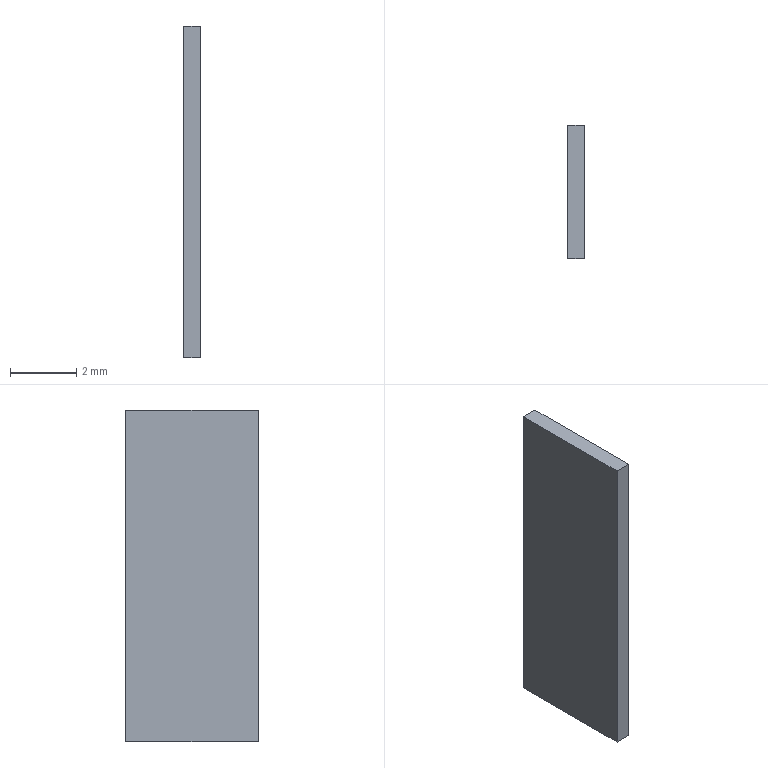Part | SolidWorks | features BaseBody 1 | 1 solid | 6 faces | box 0.5 x 4 x 10 mm | volume 20 mm3 | plane 6
STEP:
#1=CARTESIAN_POINT('',(434.6,118.75,-14.25));
#2=VERTEX_POINT('',#1);
#3=CARTESIAN_POINT('',(434.6,114.75,-14.25));
#4=VERTEX_POINT('',#3);
#5=CARTESIAN_POINT('',(434.6,86.505,-14.25));
#6=DIRECTION('',(0.,-1.,0.));
#7=VECTOR('',#6,1000.);
#8=LINE('',#5,#7);
#9=EDGE_CURVE('',#2,#4,#8,.T.);
#10=ORIENTED_EDGE('',*,*,#9,.F.);
#11=CARTESIAN_POINT('',(435.1,118.75,-14.25));
#12=VERTEX_POINT('',#11);
#13=CARTESIAN_POINT('',(435.1,118.75,-14.25));
#14=DIRECTION('',(-1.,0.,0.));
#15=VECTOR('',#14,1000.);
#16=LINE('',#13,#15);
#17=EDGE_CURVE('',#12,#2,#16,.T.);
#18=ORIENTED_EDGE('',*,*,#17,.F.);
#19=CARTESIAN_POINT('',(435.1,114.75,-14.25));
#20=VERTEX_POINT('',#19);
#21=CARTESIAN_POINT('',(435.1,86.505,-14.25));
#22=DIRECTION('',(0.,-1.,0.));
#23=VECTOR('',#22,1000.);
#24=LINE('',#21,#23);
#25=EDGE_CURVE('',#12,#20,#24,.T.);
#26=ORIENTED_EDGE('',*,*,#25,.T.);
#27=CARTESIAN_POINT('',(435.1,114.75,-14.25));
#28=DIRECTION('',(-1.,0.,0.));
#29=VECTOR('',#28,1000.);
#30=LINE('',#27,#29);
#31=EDGE_CURVE('',#20,#4,#30,.T.);
#32=ORIENTED_EDGE('',*,*,#31,.T.);
#33=EDGE_LOOP('',(#10,#18,#26,#32));
#34=FACE_OUTER_BOUND('',#33,.T.);
#35=CARTESIAN_POINT('',(435.1,86.505,-14.25));
#36=DIRECTION('',(0.,0.,-1.));
#37=DIRECTION('',(0.,1.,0.));
#38=AXIS2_PLACEMENT_3D('',#35,#36,#37);
#39=PLANE('',#38);
#40=ADVANCED_FACE('',(#34),#39,.T.);
#41=CARTESIAN_POINT('',(434.6,118.75,-4.25));
#42=VERTEX_POINT('',#41);
#43=CARTESIAN_POINT('',(434.6,118.75,0.));
#44=DIRECTION('',(0.,0.,-1.));
#45=VECTOR('',#44,1000.);
#46=LINE('',#43,#45);
#47=EDGE_CURVE('',#42,#2,#46,.T.);
#48=ORIENTED_EDGE('',*,*,#47,.F.);
#49=CARTESIAN_POINT('',(435.1,118.75,-4.25));
#50=VERTEX_POINT('',#49);
#51=CARTESIAN_POINT('',(435.1,118.75,-4.25));
#52=DIRECTION('',(-1.,0.,0.));
#53=VECTOR('',#52,1000.);
#54=LINE('',#51,#53);
#55=EDGE_CURVE('',#50,#42,#54,.T.);
#56=ORIENTED_EDGE('',*,*,#55,.F.);
#57=CARTESIAN_POINT('',(435.1,118.75,0.));
#58=DIRECTION('',(0.,0.,-1.));
#59=VECTOR('',#58,1000.);
#60=LINE('',#57,#59);
#61=EDGE_CURVE('',#50,#12,#60,.T.);
#62=ORIENTED_EDGE('',*,*,#61,.T.);
#63=ORIENTED_EDGE('',*,*,#17,.T.);
#64=EDGE_LOOP('',(#48,#56,#62,#63));
#65=FACE_OUTER_BOUND('',#64,.T.);
#66=CARTESIAN_POINT('',(435.1,118.75,0.));
#67=DIRECTION('',(0.,1.,0.));
#68=DIRECTION('',(0.,0.,1.));
#69=AXIS2_PLACEMENT_3D('',#66,#67,#68);
#70=PLANE('',#69);
#71=ADVANCED_FACE('',(#65),#70,.T.);
#72=CARTESIAN_POINT('',(434.6,114.75,-4.25));
#73=VERTEX_POINT('',#72);
#74=CARTESIAN_POINT('',(434.6,86.505,-4.25));
#75=DIRECTION('',(0.,-1.,0.));
#76=VECTOR('',#75,1000.);
#77=LINE('',#74,#76);
#78=EDGE_CURVE('',#42,#73,#77,.T.);
#79=ORIENTED_EDGE('',*,*,#78,.T.);
#80=CARTESIAN_POINT('',(435.1,114.75,-4.25));
#81=VERTEX_POINT('',#80);
#82=CARTESIAN_POINT('',(435.1,114.75,-4.25));
#83=DIRECTION('',(-1.,0.,0.));
#84=VECTOR('',#83,1000.);
#85=LINE('',#82,#84);
#86=EDGE_CURVE('',#81,#73,#85,.T.);
#87=ORIENTED_EDGE('',*,*,#86,.F.);
#88=CARTESIAN_POINT('',(435.1,86.505,-4.25));
#89=DIRECTION('',(0.,-1.,0.));
#90=VECTOR('',#89,1000.);
#91=LINE('',#88,#90);
#92=EDGE_CURVE('',#50,#81,#91,.T.);
#93=ORIENTED_EDGE('',*,*,#92,.F.);
#94=ORIENTED_EDGE('',*,*,#55,.T.);
#95=EDGE_LOOP('',(#79,#87,#93,#94));
#96=FACE_OUTER_BOUND('',#95,.T.);
#97=CARTESIAN_POINT('',(435.1,86.505,-4.25));
#98=DIRECTION('',(0.,0.,-1.));
#99=DIRECTION('',(-1.,0.,0.));
#100=AXIS2_PLACEMENT_3D('',#97,#98,#99);
#101=PLANE('',#100);
#102=ADVANCED_FACE('',(#96),#101,.F.);
#103=CARTESIAN_POINT('',(434.6,114.75,0.));
#104=DIRECTION('',(0.,0.,-1.));
#105=VECTOR('',#104,1000.);
#106=LINE('',#103,#105);
#107=EDGE_CURVE('',#73,#4,#106,.T.);
#108=ORIENTED_EDGE('',*,*,#107,.T.);
#109=ORIENTED_EDGE('',*,*,#31,.F.);
#110=CARTESIAN_POINT('',(435.1,114.75,0.));
#111=DIRECTION('',(0.,0.,-1.));
#112=VECTOR('',#111,1000.);
#113=LINE('',#110,#112);
#114=EDGE_CURVE('',#81,#20,#113,.T.);
#115=ORIENTED_EDGE('',*,*,#114,.F.);
#116=ORIENTED_EDGE('',*,*,#86,.T.);
#117=EDGE_LOOP('',(#108,#109,#115,#116));
#118=FACE_OUTER_BOUND('',#117,.T.);
#119=CARTESIAN_POINT('',(435.1,114.75,0.));
#120=DIRECTION('',(0.,1.,0.));
#121=DIRECTION('',(0.,0.,1.));
#122=AXIS2_PLACEMENT_3D('',#119,#120,#121);
#123=PLANE('',#122);
#124=ADVANCED_FACE('',(#118),#123,.F.);
#125=ORIENTED_EDGE('',*,*,#25,.F.);
#126=ORIENTED_EDGE('',*,*,#61,.F.);
#127=ORIENTED_EDGE('',*,*,#92,.T.);
#128=ORIENTED_EDGE('',*,*,#114,.T.);
#129=EDGE_LOOP('',(#125,#126,#127,#128));
#130=FACE_OUTER_BOUND('',#129,.T.);
#131=CARTESIAN_POINT('',(435.1,86.505,0.));
#132=DIRECTION('',(1.,0.,0.));
#133=DIRECTION('',(0.,0.,-1.));
#134=AXIS2_PLACEMENT_3D('',#131,#132,#133);
#135=PLANE('',#134);
#136=ADVANCED_FACE('',(#130),#135,.T.);
#137=ORIENTED_EDGE('',*,*,#9,.T.);
#138=ORIENTED_EDGE('',*,*,#107,.F.);
#139=ORIENTED_EDGE('',*,*,#78,.F.);
#140=ORIENTED_EDGE('',*,*,#47,.T.);
#141=EDGE_LOOP('',(#137,#138,#139,#140));
#142=FACE_OUTER_BOUND('',#141,.T.);
#143=CARTESIAN_POINT('',(434.6,86.505,0.));
#144=DIRECTION('',(1.,0.,0.));
#145=DIRECTION('',(0.,0.,-1.));
#146=AXIS2_PLACEMENT_3D('',#143,#144,#145);
#147=PLANE('',#146);
#148=ADVANCED_FACE('',(#142),#147,.F.);
#149=CLOSED_SHELL('',(#40,#71,#102,#124,#136,#148));
#150=MANIFOLD_SOLID_BREP('',#149);
#151=CARTESIAN_POINT('',(0.,0.,0.));
#152=DIRECTION('',(0.,0.,1.));
#153=DIRECTION('',(1.,0.,0.));
#154=AXIS2_PLACEMENT_3D('',#151,#152,#153);
#155=(LENGTH_UNIT()NAMED_UNIT(*)SI_UNIT(.MILLI.,.METRE.));
#156=UNCERTAINTY_MEASURE_WITH_UNIT(LENGTH_MEASURE(0.00001),#155,'','');
#157=(NAMED_UNIT(*)PLANE_ANGLE_UNIT()SI_UNIT($,.RADIAN.));
#158=(NAMED_UNIT(*)SI_UNIT($,.STERADIAN.)SOLID_ANGLE_UNIT());
#159=(GEOMETRIC_REPRESENTATION_CONTEXT(3)GLOBAL_UNCERTAINTY_ASSIGNED_CONTEXT((#156))GLOBAL_UNIT_ASSIGNED_CONTEXT((#155,#157,#158))REPRESENTATION_CONTEXT('',''));
#160=ADVANCED_BREP_SHAPE_REPRESENTATION('',(#150,#154),#159);